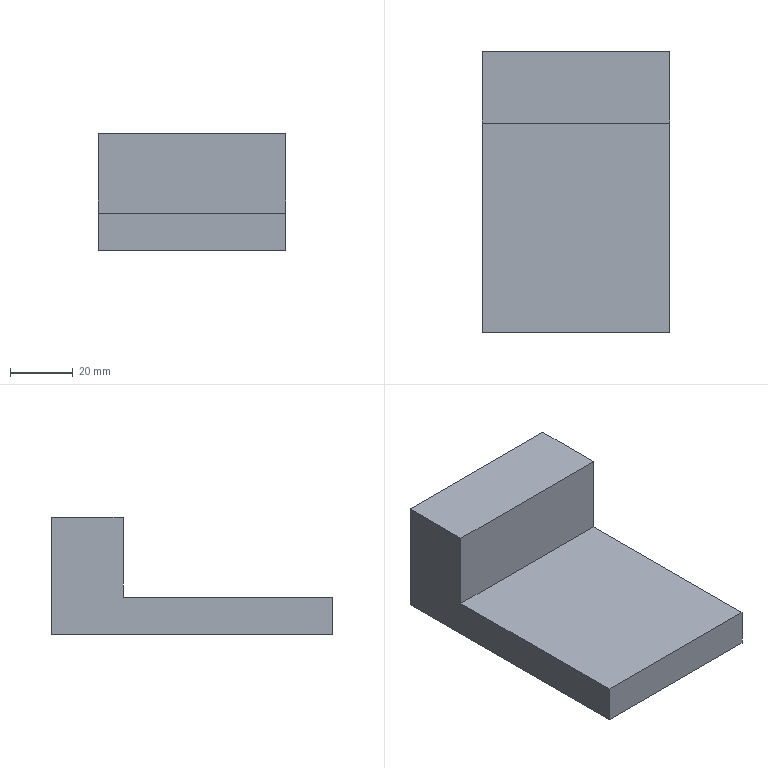Part | STEP file | 001-010-Waste slider connecting plate | 1 solid | 8 faces | box 60 x 90 x 37.5 mm | volume 99990 mm3 | plane 8
STEP:
#1=CARTESIAN_POINT('',(0.,0.,0.));
#2=DIRECTION('',(0.,0.,1.));
#3=DIRECTION('',(1.,0.,0.));
#4=AXIS2_PLACEMENT_3D('',#1,#2,#3);
#5=CARTESIAN_POINT('',(30.,22.,37.5));
#6=VERTEX_POINT('',#5);
#7=CARTESIAN_POINT('',(30.,45.,37.5));
#8=VERTEX_POINT('',#7);
#9=CARTESIAN_POINT('',(30.,-45.,37.5));
#10=DIRECTION('',(0.,1.,0.));
#11=VECTOR('',#10,1.);
#12=LINE('',#9,#11);
#13=CARTESIAN_POINT('',(30.,-45.,37.5));
#14=DIRECTION('',(-1.,0.,0.));
#15=DIRECTION('',(0.,-1.,0.));
#16=AXIS2_PLACEMENT_3D('',#13,#14,#15);
#17=PLANE('',#16);
#18=CARTESIAN_POINT('',(0.,0.));
#19=DIRECTION('',(-1.,0.));
#20=VECTOR('',#19,1.);
#21=LINE('',#18,#20);
#22=(GEOMETRIC_REPRESENTATION_CONTEXT(2)PARAMETRIC_REPRESENTATION_CONTEXT()REPRESENTATION_CONTEXT('',''));
#23=DEFINITIONAL_REPRESENTATION('',(#21),#22);
#24=PCURVE('',#17,#23);
#25=CARTESIAN_POINT('',(0.,0.,37.5));
#26=DIRECTION('',(0.,0.,-1.));
#27=DIRECTION('',(-1.,0.,0.));
#28=AXIS2_PLACEMENT_3D('',#25,#26,#27);
#29=PLANE('',#28);
#30=CARTESIAN_POINT('',(-30.,-45.));
#31=DIRECTION('',(0.,1.));
#32=VECTOR('',#31,1.);
#33=LINE('',#30,#32);
#34=(GEOMETRIC_REPRESENTATION_CONTEXT(2)PARAMETRIC_REPRESENTATION_CONTEXT()REPRESENTATION_CONTEXT('',''));
#35=DEFINITIONAL_REPRESENTATION('',(#33),#34);
#36=PCURVE('',#29,#35);
#37=SURFACE_CURVE('',#12,(#24,#36),.PCURVE_S1.);
#38=EDGE_CURVE('',#6,#8,#37,.T.);
#39=ORIENTED_EDGE('',*,*,#38,.F.);
#40=CARTESIAN_POINT('',(30.,22.,12.));
#41=VERTEX_POINT('',#40);
#42=CARTESIAN_POINT('',(30.,22.,37.5));
#43=DIRECTION('',(0.,0.,1.));
#44=VECTOR('',#43,1.);
#45=LINE('',#42,#44);
#46=CARTESIAN_POINT('',(-67.,0.));
#47=DIRECTION('',(0.,1.));
#48=VECTOR('',#47,1.);
#49=LINE('',#46,#48);
#50=(GEOMETRIC_REPRESENTATION_CONTEXT(2)PARAMETRIC_REPRESENTATION_CONTEXT()REPRESENTATION_CONTEXT('',''));
#51=DEFINITIONAL_REPRESENTATION('',(#49),#50);
#52=PCURVE('',#17,#51);
#53=CARTESIAN_POINT('',(-30.,22.,37.5));
#54=DIRECTION('',(0.,1.,0.));
#55=DIRECTION('',(-1.,0.,0.));
#56=AXIS2_PLACEMENT_3D('',#53,#54,#55);
#57=PLANE('',#56);
#58=CARTESIAN_POINT('',(-60.,0.));
#59=DIRECTION('',(0.,1.));
#60=VECTOR('',#59,1.);
#61=LINE('',#58,#60);
#62=(GEOMETRIC_REPRESENTATION_CONTEXT(2)PARAMETRIC_REPRESENTATION_CONTEXT()REPRESENTATION_CONTEXT('',''));
#63=DEFINITIONAL_REPRESENTATION('',(#61),#62);
#64=PCURVE('',#57,#63);
#65=SURFACE_CURVE('',#45,(#52,#64),.PCURVE_S1.);
#66=EDGE_CURVE('',#41,#6,#65,.T.);
#67=ORIENTED_EDGE('',*,*,#66,.F.);
#68=CARTESIAN_POINT('',(30.,-45.,12.));
#69=VERTEX_POINT('',#68);
#70=CARTESIAN_POINT('',(30.,-45.,12.));
#71=DIRECTION('',(0.,1.,0.));
#72=VECTOR('',#71,1.);
#73=LINE('',#70,#72);
#74=CARTESIAN_POINT('',(0.,-25.5));
#75=DIRECTION('',(-1.,0.));
#76=VECTOR('',#75,1.);
#77=LINE('',#74,#76);
#78=(GEOMETRIC_REPRESENTATION_CONTEXT(2)PARAMETRIC_REPRESENTATION_CONTEXT()REPRESENTATION_CONTEXT('',''));
#79=DEFINITIONAL_REPRESENTATION('',(#77),#78);
#80=PCURVE('',#17,#79);
#81=CARTESIAN_POINT('',(-30.,-45.,12.));
#82=DIRECTION('',(0.,0.,-1.));
#83=DIRECTION('',(-1.,0.,0.));
#84=AXIS2_PLACEMENT_3D('',#81,#82,#83);
#85=PLANE('',#84);
#86=CARTESIAN_POINT('',(-60.,0.));
#87=DIRECTION('',(0.,1.));
#88=VECTOR('',#87,1.);
#89=LINE('',#86,#88);
#90=(GEOMETRIC_REPRESENTATION_CONTEXT(2)PARAMETRIC_REPRESENTATION_CONTEXT()REPRESENTATION_CONTEXT('',''));
#91=DEFINITIONAL_REPRESENTATION('',(#89),#90);
#92=PCURVE('',#85,#91);
#93=SURFACE_CURVE('',#73,(#80,#92),.PCURVE_S1.);
#94=EDGE_CURVE('',#69,#41,#93,.T.);
#95=ORIENTED_EDGE('',*,*,#94,.F.);
#96=CARTESIAN_POINT('',(30.,-45.,0.));
#97=VERTEX_POINT('',#96);
#98=CARTESIAN_POINT('',(30.,-45.,37.5));
#99=DIRECTION('',(0.,0.,-1.));
#100=VECTOR('',#99,1.);
#101=LINE('',#98,#100);
#102=CARTESIAN_POINT('',(0.,0.));
#103=DIRECTION('',(0.,-1.));
#104=VECTOR('',#103,1.);
#105=LINE('',#102,#104);
#106=(GEOMETRIC_REPRESENTATION_CONTEXT(2)PARAMETRIC_REPRESENTATION_CONTEXT()REPRESENTATION_CONTEXT('',''));
#107=DEFINITIONAL_REPRESENTATION('',(#105),#106);
#108=PCURVE('',#17,#107);
#109=CARTESIAN_POINT('',(-30.,-45.,37.5));
#110=DIRECTION('',(0.,1.,0.));
#111=DIRECTION('',(0.,0.,1.));
#112=AXIS2_PLACEMENT_3D('',#109,#110,#111);
#113=PLANE('',#112);
#114=CARTESIAN_POINT('',(0.,60.));
#115=DIRECTION('',(-1.,0.));
#116=VECTOR('',#115,1.);
#117=LINE('',#114,#116);
#118=(GEOMETRIC_REPRESENTATION_CONTEXT(2)PARAMETRIC_REPRESENTATION_CONTEXT()REPRESENTATION_CONTEXT('',''));
#119=DEFINITIONAL_REPRESENTATION('',(#117),#118);
#120=PCURVE('',#113,#119);
#121=SURFACE_CURVE('',#101,(#108,#120),.PCURVE_S1.);
#122=EDGE_CURVE('',#69,#97,#121,.T.);
#123=ORIENTED_EDGE('',*,*,#122,.T.);
#124=CARTESIAN_POINT('',(30.,45.,0.));
#125=VERTEX_POINT('',#124);
#126=CARTESIAN_POINT('',(30.,-45.,0.));
#127=DIRECTION('',(0.,1.,0.));
#128=VECTOR('',#127,1.);
#129=LINE('',#126,#128);
#130=CARTESIAN_POINT('',(0.,-37.5));
#131=DIRECTION('',(-1.,0.));
#132=VECTOR('',#131,1.);
#133=LINE('',#130,#132);
#134=(GEOMETRIC_REPRESENTATION_CONTEXT(2)PARAMETRIC_REPRESENTATION_CONTEXT()REPRESENTATION_CONTEXT('',''));
#135=DEFINITIONAL_REPRESENTATION('',(#133),#134);
#136=PCURVE('',#17,#135);
#137=CARTESIAN_POINT('',(0.,0.,0.));
#138=DIRECTION('',(0.,0.,-1.));
#139=DIRECTION('',(-1.,0.,0.));
#140=AXIS2_PLACEMENT_3D('',#137,#138,#139);
#141=PLANE('',#140);
#142=CARTESIAN_POINT('',(-30.,-45.));
#143=DIRECTION('',(0.,1.));
#144=VECTOR('',#143,1.);
#145=LINE('',#142,#144);
#146=(GEOMETRIC_REPRESENTATION_CONTEXT(2)PARAMETRIC_REPRESENTATION_CONTEXT()REPRESENTATION_CONTEXT('',''));
#147=DEFINITIONAL_REPRESENTATION('',(#145),#146);
#148=PCURVE('',#141,#147);
#149=SURFACE_CURVE('',#129,(#136,#148),.PCURVE_S1.);
#150=EDGE_CURVE('',#97,#125,#149,.T.);
#151=ORIENTED_EDGE('',*,*,#150,.T.);
#152=CARTESIAN_POINT('',(30.,45.,37.5));
#153=DIRECTION('',(0.,0.,-1.));
#154=VECTOR('',#153,1.);
#155=LINE('',#152,#154);
#156=CARTESIAN_POINT('',(-90.,0.));
#157=DIRECTION('',(0.,-1.));
#158=VECTOR('',#157,1.);
#159=LINE('',#156,#158);
#160=(GEOMETRIC_REPRESENTATION_CONTEXT(2)PARAMETRIC_REPRESENTATION_CONTEXT()REPRESENTATION_CONTEXT('',''));
#161=DEFINITIONAL_REPRESENTATION('',(#159),#160);
#162=PCURVE('',#17,#161);
#163=CARTESIAN_POINT('',(-30.,45.,37.5));
#164=DIRECTION('',(0.,-1.,0.));
#165=DIRECTION('',(1.,0.,0.));
#166=AXIS2_PLACEMENT_3D('',#163,#164,#165);
#167=PLANE('',#166);
#168=CARTESIAN_POINT('',(60.,0.));
#169=DIRECTION('',(0.,-1.));
#170=VECTOR('',#169,1.);
#171=LINE('',#168,#170);
#172=(GEOMETRIC_REPRESENTATION_CONTEXT(2)PARAMETRIC_REPRESENTATION_CONTEXT()REPRESENTATION_CONTEXT('',''));
#173=DEFINITIONAL_REPRESENTATION('',(#171),#172);
#174=PCURVE('',#167,#173);
#175=SURFACE_CURVE('',#155,(#162,#174),.PCURVE_S1.);
#176=EDGE_CURVE('',#8,#125,#175,.T.);
#177=ORIENTED_EDGE('',*,*,#176,.F.);
#178=EDGE_LOOP('',(#39,#67,#95,#123,#151,#177));
#179=FACE_BOUND('',#178,.T.);
#180=ADVANCED_FACE('',(#179),#17,.F.);
#181=CARTESIAN_POINT('',(-30.,45.,0.));
#182=VERTEX_POINT('',#181);
#183=CARTESIAN_POINT('',(-30.,45.,0.));
#184=DIRECTION('',(-1.,0.,0.));
#185=VECTOR('',#184,1.);
#186=LINE('',#183,#185);
#187=CARTESIAN_POINT('',(0.,-37.5));
#188=DIRECTION('',(-1.,0.));
#189=VECTOR('',#188,1.);
#190=LINE('',#187,#189);
#191=(GEOMETRIC_REPRESENTATION_CONTEXT(2)PARAMETRIC_REPRESENTATION_CONTEXT()REPRESENTATION_CONTEXT('',''));
#192=DEFINITIONAL_REPRESENTATION('',(#190),#191);
#193=PCURVE('',#167,#192);
#194=CARTESIAN_POINT('',(30.,45.));
#195=DIRECTION('',(1.,0.));
#196=VECTOR('',#195,1.);
#197=LINE('',#194,#196);
#198=(GEOMETRIC_REPRESENTATION_CONTEXT(2)PARAMETRIC_REPRESENTATION_CONTEXT()REPRESENTATION_CONTEXT('',''));
#199=DEFINITIONAL_REPRESENTATION('',(#197),#198);
#200=PCURVE('',#141,#199);
#201=SURFACE_CURVE('',#186,(#193,#200),.PCURVE_S1.);
#202=EDGE_CURVE('',#125,#182,#201,.T.);
#203=ORIENTED_EDGE('',*,*,#202,.T.);
#204=CARTESIAN_POINT('',(-30.,45.,37.5));
#205=VERTEX_POINT('',#204);
#206=CARTESIAN_POINT('',(-30.,45.,37.5));
#207=DIRECTION('',(0.,0.,-1.));
#208=VECTOR('',#207,1.);
#209=LINE('',#206,#208);
#210=CARTESIAN_POINT('',(0.,0.));
#211=DIRECTION('',(0.,-1.));
#212=VECTOR('',#211,1.);
#213=LINE('',#210,#212);
#214=(GEOMETRIC_REPRESENTATION_CONTEXT(2)PARAMETRIC_REPRESENTATION_CONTEXT()REPRESENTATION_CONTEXT('',''));
#215=DEFINITIONAL_REPRESENTATION('',(#213),#214);
#216=PCURVE('',#167,#215);
#217=CARTESIAN_POINT('',(-30.,-45.,37.5));
#218=DIRECTION('',(1.,0.,0.));
#219=DIRECTION('',(0.,0.,-1.));
#220=AXIS2_PLACEMENT_3D('',#217,#218,#219);
#221=PLANE('',#220);
#222=CARTESIAN_POINT('',(0.,90.));
#223=DIRECTION('',(1.,0.));
#224=VECTOR('',#223,1.);
#225=LINE('',#222,#224);
#226=(GEOMETRIC_REPRESENTATION_CONTEXT(2)PARAMETRIC_REPRESENTATION_CONTEXT()REPRESENTATION_CONTEXT('',''));
#227=DEFINITIONAL_REPRESENTATION('',(#225),#226);
#228=PCURVE('',#221,#227);
#229=SURFACE_CURVE('',#209,(#216,#228),.PCURVE_S1.);
#230=EDGE_CURVE('',#205,#182,#229,.T.);
#231=ORIENTED_EDGE('',*,*,#230,.F.);
#232=CARTESIAN_POINT('',(-30.,45.,37.5));
#233=DIRECTION('',(-1.,0.,0.));
#234=VECTOR('',#233,1.);
#235=LINE('',#232,#234);
#236=CARTESIAN_POINT('',(0.,0.));
#237=DIRECTION('',(-1.,0.));
#238=VECTOR('',#237,1.);
#239=LINE('',#236,#238);
#240=(GEOMETRIC_REPRESENTATION_CONTEXT(2)PARAMETRIC_REPRESENTATION_CONTEXT()REPRESENTATION_CONTEXT('',''));
#241=DEFINITIONAL_REPRESENTATION('',(#239),#240);
#242=PCURVE('',#167,#241);
#243=CARTESIAN_POINT('',(30.,45.));
#244=DIRECTION('',(1.,0.));
#245=VECTOR('',#244,1.);
#246=LINE('',#243,#245);
#247=(GEOMETRIC_REPRESENTATION_CONTEXT(2)PARAMETRIC_REPRESENTATION_CONTEXT()REPRESENTATION_CONTEXT('',''));
#248=DEFINITIONAL_REPRESENTATION('',(#246),#247);
#249=PCURVE('',#29,#248);
#250=SURFACE_CURVE('',#235,(#242,#249),.PCURVE_S1.);
#251=EDGE_CURVE('',#8,#205,#250,.T.);
#252=ORIENTED_EDGE('',*,*,#251,.F.);
#253=ORIENTED_EDGE('',*,*,#176,.T.);
#254=EDGE_LOOP('',(#203,#231,#252,#253));
#255=FACE_BOUND('',#254,.T.);
#256=ADVANCED_FACE('',(#255),#167,.F.);
#257=CARTESIAN_POINT('',(-30.,-45.,12.));
#258=VERTEX_POINT('',#257);
#259=CARTESIAN_POINT('',(-30.,22.,12.));
#260=VERTEX_POINT('',#259);
#261=CARTESIAN_POINT('',(-30.,-45.,12.));
#262=DIRECTION('',(0.,1.,0.));
#263=VECTOR('',#262,1.);
#264=LINE('',#261,#263);
#265=CARTESIAN_POINT('',(25.5,0.));
#266=DIRECTION('',(0.,1.));
#267=VECTOR('',#266,1.);
#268=LINE('',#265,#267);
#269=(GEOMETRIC_REPRESENTATION_CONTEXT(2)PARAMETRIC_REPRESENTATION_CONTEXT()REPRESENTATION_CONTEXT('',''));
#270=DEFINITIONAL_REPRESENTATION('',(#268),#269);
#271=PCURVE('',#221,#270);
#272=CARTESIAN_POINT('',(0.,0.));
#273=DIRECTION('',(0.,1.));
#274=VECTOR('',#273,1.);
#275=LINE('',#272,#274);
#276=(GEOMETRIC_REPRESENTATION_CONTEXT(2)PARAMETRIC_REPRESENTATION_CONTEXT()REPRESENTATION_CONTEXT('',''));
#277=DEFINITIONAL_REPRESENTATION('',(#275),#276);
#278=PCURVE('',#85,#277);
#279=SURFACE_CURVE('',#264,(#271,#278),.PCURVE_S1.);
#280=EDGE_CURVE('',#258,#260,#279,.T.);
#281=ORIENTED_EDGE('',*,*,#280,.T.);
#282=CARTESIAN_POINT('',(-30.,22.,37.5));
#283=VERTEX_POINT('',#282);
#284=CARTESIAN_POINT('',(-30.,22.,37.5));
#285=DIRECTION('',(0.,0.,1.));
#286=VECTOR('',#285,1.);
#287=LINE('',#284,#286);
#288=CARTESIAN_POINT('',(0.,67.));
#289=DIRECTION('',(-1.,0.));
#290=VECTOR('',#289,1.);
#291=LINE('',#288,#290);
#292=(GEOMETRIC_REPRESENTATION_CONTEXT(2)PARAMETRIC_REPRESENTATION_CONTEXT()REPRESENTATION_CONTEXT('',''));
#293=DEFINITIONAL_REPRESENTATION('',(#291),#292);
#294=PCURVE('',#221,#293);
#295=CARTESIAN_POINT('',(0.,0.));
#296=DIRECTION('',(0.,1.));
#297=VECTOR('',#296,1.);
#298=LINE('',#295,#297);
#299=(GEOMETRIC_REPRESENTATION_CONTEXT(2)PARAMETRIC_REPRESENTATION_CONTEXT()REPRESENTATION_CONTEXT('',''));
#300=DEFINITIONAL_REPRESENTATION('',(#298),#299);
#301=PCURVE('',#57,#300);
#302=SURFACE_CURVE('',#287,(#294,#301),.PCURVE_S1.);
#303=EDGE_CURVE('',#260,#283,#302,.T.);
#304=ORIENTED_EDGE('',*,*,#303,.T.);
#305=CARTESIAN_POINT('',(-30.,-45.,37.5));
#306=DIRECTION('',(0.,-1.,0.));
#307=VECTOR('',#306,1.);
#308=LINE('',#305,#307);
#309=CARTESIAN_POINT('',(0.,0.));
#310=DIRECTION('',(0.,-1.));
#311=VECTOR('',#310,1.);
#312=LINE('',#309,#311);
#313=(GEOMETRIC_REPRESENTATION_CONTEXT(2)PARAMETRIC_REPRESENTATION_CONTEXT()REPRESENTATION_CONTEXT('',''));
#314=DEFINITIONAL_REPRESENTATION('',(#312),#313);
#315=PCURVE('',#221,#314);
#316=CARTESIAN_POINT('',(30.,-45.));
#317=DIRECTION('',(0.,-1.));
#318=VECTOR('',#317,1.);
#319=LINE('',#316,#318);
#320=(GEOMETRIC_REPRESENTATION_CONTEXT(2)PARAMETRIC_REPRESENTATION_CONTEXT()REPRESENTATION_CONTEXT('',''));
#321=DEFINITIONAL_REPRESENTATION('',(#319),#320);
#322=PCURVE('',#29,#321);
#323=SURFACE_CURVE('',#308,(#315,#322),.PCURVE_S1.);
#324=EDGE_CURVE('',#205,#283,#323,.T.);
#325=ORIENTED_EDGE('',*,*,#324,.F.);
#326=ORIENTED_EDGE('',*,*,#230,.T.);
#327=CARTESIAN_POINT('',(-30.,-45.,0.));
#328=VERTEX_POINT('',#327);
#329=CARTESIAN_POINT('',(-30.,-45.,0.));
#330=DIRECTION('',(0.,-1.,0.));
#331=VECTOR('',#330,1.);
#332=LINE('',#329,#331);
#333=CARTESIAN_POINT('',(37.5,0.));
#334=DIRECTION('',(0.,-1.));
#335=VECTOR('',#334,1.);
#336=LINE('',#333,#335);
#337=(GEOMETRIC_REPRESENTATION_CONTEXT(2)PARAMETRIC_REPRESENTATION_CONTEXT()REPRESENTATION_CONTEXT('',''));
#338=DEFINITIONAL_REPRESENTATION('',(#336),#337);
#339=PCURVE('',#221,#338);
#340=CARTESIAN_POINT('',(30.,-45.));
#341=DIRECTION('',(0.,-1.));
#342=VECTOR('',#341,1.);
#343=LINE('',#340,#342);
#344=(GEOMETRIC_REPRESENTATION_CONTEXT(2)PARAMETRIC_REPRESENTATION_CONTEXT()REPRESENTATION_CONTEXT('',''));
#345=DEFINITIONAL_REPRESENTATION('',(#343),#344);
#346=PCURVE('',#141,#345);
#347=SURFACE_CURVE('',#332,(#339,#346),.PCURVE_S1.);
#348=EDGE_CURVE('',#182,#328,#347,.T.);
#349=ORIENTED_EDGE('',*,*,#348,.T.);
#350=CARTESIAN_POINT('',(-30.,-45.,37.5));
#351=DIRECTION('',(0.,0.,-1.));
#352=VECTOR('',#351,1.);
#353=LINE('',#350,#352);
#354=CARTESIAN_POINT('',(0.,0.));
#355=DIRECTION('',(1.,0.));
#356=VECTOR('',#355,1.);
#357=LINE('',#354,#356);
#358=(GEOMETRIC_REPRESENTATION_CONTEXT(2)PARAMETRIC_REPRESENTATION_CONTEXT()REPRESENTATION_CONTEXT('',''));
#359=DEFINITIONAL_REPRESENTATION('',(#357),#358);
#360=PCURVE('',#221,#359);
#361=CARTESIAN_POINT('',(0.,0.));
#362=DIRECTION('',(-1.,0.));
#363=VECTOR('',#362,1.);
#364=LINE('',#361,#363);
#365=(GEOMETRIC_REPRESENTATION_CONTEXT(2)PARAMETRIC_REPRESENTATION_CONTEXT()REPRESENTATION_CONTEXT('',''));
#366=DEFINITIONAL_REPRESENTATION('',(#364),#365);
#367=PCURVE('',#113,#366);
#368=SURFACE_CURVE('',#353,(#360,#367),.PCURVE_S1.);
#369=EDGE_CURVE('',#258,#328,#368,.T.);
#370=ORIENTED_EDGE('',*,*,#369,.F.);
#371=EDGE_LOOP('',(#281,#304,#325,#326,#349,#370));
#372=FACE_BOUND('',#371,.T.);
#373=ADVANCED_FACE('',(#372),#221,.F.);
#374=ORIENTED_EDGE('',*,*,#122,.F.);
#375=CARTESIAN_POINT('',(-30.,-45.,12.));
#376=DIRECTION('',(1.,0.,0.));
#377=VECTOR('',#376,1.);
#378=LINE('',#375,#377);
#379=CARTESIAN_POINT('',(-25.5,0.));
#380=DIRECTION('',(0.,1.));
#381=VECTOR('',#380,1.);
#382=LINE('',#379,#381);
#383=(GEOMETRIC_REPRESENTATION_CONTEXT(2)PARAMETRIC_REPRESENTATION_CONTEXT()REPRESENTATION_CONTEXT('',''));
#384=DEFINITIONAL_REPRESENTATION('',(#382),#383);
#385=PCURVE('',#113,#384);
#386=CARTESIAN_POINT('',(0.,0.));
#387=DIRECTION('',(-1.,0.));
#388=VECTOR('',#387,1.);
#389=LINE('',#386,#388);
#390=(GEOMETRIC_REPRESENTATION_CONTEXT(2)PARAMETRIC_REPRESENTATION_CONTEXT()REPRESENTATION_CONTEXT('',''));
#391=DEFINITIONAL_REPRESENTATION('',(#389),#390);
#392=PCURVE('',#85,#391);
#393=SURFACE_CURVE('',#378,(#385,#392),.PCURVE_S1.);
#394=EDGE_CURVE('',#258,#69,#393,.T.);
#395=ORIENTED_EDGE('',*,*,#394,.F.);
#396=ORIENTED_EDGE('',*,*,#369,.T.);
#397=CARTESIAN_POINT('',(-30.,-45.,0.));
#398=DIRECTION('',(1.,0.,0.));
#399=VECTOR('',#398,1.);
#400=LINE('',#397,#399);
#401=CARTESIAN_POINT('',(-37.5,0.));
#402=DIRECTION('',(0.,1.));
#403=VECTOR('',#402,1.);
#404=LINE('',#401,#403);
#405=(GEOMETRIC_REPRESENTATION_CONTEXT(2)PARAMETRIC_REPRESENTATION_CONTEXT()REPRESENTATION_CONTEXT('',''));
#406=DEFINITIONAL_REPRESENTATION('',(#404),#405);
#407=PCURVE('',#113,#406);
#408=CARTESIAN_POINT('',(30.,-45.));
#409=DIRECTION('',(-1.,0.));
#410=VECTOR('',#409,1.);
#411=LINE('',#408,#410);
#412=(GEOMETRIC_REPRESENTATION_CONTEXT(2)PARAMETRIC_REPRESENTATION_CONTEXT()REPRESENTATION_CONTEXT('',''));
#413=DEFINITIONAL_REPRESENTATION('',(#411),#412);
#414=PCURVE('',#141,#413);
#415=SURFACE_CURVE('',#400,(#407,#414),.PCURVE_S1.);
#416=EDGE_CURVE('',#328,#97,#415,.T.);
#417=ORIENTED_EDGE('',*,*,#416,.T.);
#418=EDGE_LOOP('',(#374,#395,#396,#417));
#419=FACE_BOUND('',#418,.T.);
#420=ADVANCED_FACE('',(#419),#113,.F.);
#421=ORIENTED_EDGE('',*,*,#324,.T.);
#422=CARTESIAN_POINT('',(-30.,22.,37.5));
#423=DIRECTION('',(1.,0.,0.));
#424=VECTOR('',#423,1.);
#425=LINE('',#422,#424);
#426=CARTESIAN_POINT('',(30.,22.));
#427=DIRECTION('',(-1.,0.));
#428=VECTOR('',#427,1.);
#429=LINE('',#426,#428);
#430=(GEOMETRIC_REPRESENTATION_CONTEXT(2)PARAMETRIC_REPRESENTATION_CONTEXT()REPRESENTATION_CONTEXT('',''));
#431=DEFINITIONAL_REPRESENTATION('',(#429),#430);
#432=PCURVE('',#29,#431);
#433=CARTESIAN_POINT('',(0.,0.));
#434=DIRECTION('',(-1.,0.));
#435=VECTOR('',#434,1.);
#436=LINE('',#433,#435);
#437=(GEOMETRIC_REPRESENTATION_CONTEXT(2)PARAMETRIC_REPRESENTATION_CONTEXT()REPRESENTATION_CONTEXT('',''));
#438=DEFINITIONAL_REPRESENTATION('',(#436),#437);
#439=PCURVE('',#57,#438);
#440=SURFACE_CURVE('',#425,(#432,#439),.PCURVE_S1.);
#441=EDGE_CURVE('',#283,#6,#440,.T.);
#442=ORIENTED_EDGE('',*,*,#441,.T.);
#443=ORIENTED_EDGE('',*,*,#38,.T.);
#444=ORIENTED_EDGE('',*,*,#251,.T.);
#445=EDGE_LOOP('',(#421,#442,#443,#444));
#446=FACE_BOUND('',#445,.T.);
#447=ADVANCED_FACE('',(#446),#29,.F.);
#448=ORIENTED_EDGE('',*,*,#150,.F.);
#449=ORIENTED_EDGE('',*,*,#416,.F.);
#450=ORIENTED_EDGE('',*,*,#348,.F.);
#451=ORIENTED_EDGE('',*,*,#202,.F.);
#452=EDGE_LOOP('',(#448,#449,#450,#451));
#453=FACE_BOUND('',#452,.T.);
#454=ADVANCED_FACE('',(#453),#141,.T.);
#455=ORIENTED_EDGE('',*,*,#66,.T.);
#456=ORIENTED_EDGE('',*,*,#441,.F.);
#457=ORIENTED_EDGE('',*,*,#303,.F.);
#458=CARTESIAN_POINT('',(-30.,22.,12.));
#459=DIRECTION('',(1.,0.,0.));
#460=VECTOR('',#459,1.);
#461=LINE('',#458,#460);
#462=CARTESIAN_POINT('',(0.,-25.5));
#463=DIRECTION('',(-1.,0.));
#464=VECTOR('',#463,1.);
#465=LINE('',#462,#464);
#466=(GEOMETRIC_REPRESENTATION_CONTEXT(2)PARAMETRIC_REPRESENTATION_CONTEXT()REPRESENTATION_CONTEXT('',''));
#467=DEFINITIONAL_REPRESENTATION('',(#465),#466);
#468=PCURVE('',#57,#467);
#469=CARTESIAN_POINT('',(0.,67.));
#470=DIRECTION('',(-1.,0.));
#471=VECTOR('',#470,1.);
#472=LINE('',#469,#471);
#473=(GEOMETRIC_REPRESENTATION_CONTEXT(2)PARAMETRIC_REPRESENTATION_CONTEXT()REPRESENTATION_CONTEXT('',''));
#474=DEFINITIONAL_REPRESENTATION('',(#472),#473);
#475=PCURVE('',#85,#474);
#476=SURFACE_CURVE('',#461,(#468,#475),.PCURVE_S1.);
#477=EDGE_CURVE('',#260,#41,#476,.T.);
#478=ORIENTED_EDGE('',*,*,#477,.T.);
#479=EDGE_LOOP('',(#455,#456,#457,#478));
#480=FACE_BOUND('',#479,.T.);
#481=ADVANCED_FACE('',(#480),#57,.F.);
#482=ORIENTED_EDGE('',*,*,#94,.T.);
#483=ORIENTED_EDGE('',*,*,#477,.F.);
#484=ORIENTED_EDGE('',*,*,#280,.F.);
#485=ORIENTED_EDGE('',*,*,#394,.T.);
#486=EDGE_LOOP('',(#482,#483,#484,#485));
#487=FACE_BOUND('',#486,.T.);
#488=ADVANCED_FACE('',(#487),#85,.F.);
#489=CLOSED_SHELL('',(#180,#256,#373,#420,#447,#454,#481,#488));
#490=MANIFOLD_SOLID_BREP('',#489);
#491=(LENGTH_UNIT()NAMED_UNIT(*)SI_UNIT(.MILLI.,.METRE.));
#492=UNCERTAINTY_MEASURE_WITH_UNIT(LENGTH_MEASURE(0.0000001),#491,'','');
#493=(NAMED_UNIT(*)PLANE_ANGLE_UNIT()SI_UNIT($,.RADIAN.));
#494=(NAMED_UNIT(*)SI_UNIT($,.STERADIAN.)SOLID_ANGLE_UNIT());
#495=(GEOMETRIC_REPRESENTATION_CONTEXT(3)GLOBAL_UNCERTAINTY_ASSIGNED_CONTEXT((#492))GLOBAL_UNIT_ASSIGNED_CONTEXT((#491,#493,#494))REPRESENTATION_CONTEXT('',''));
#496=ADVANCED_BREP_SHAPE_REPRESENTATION('',(#4,#490),#495);